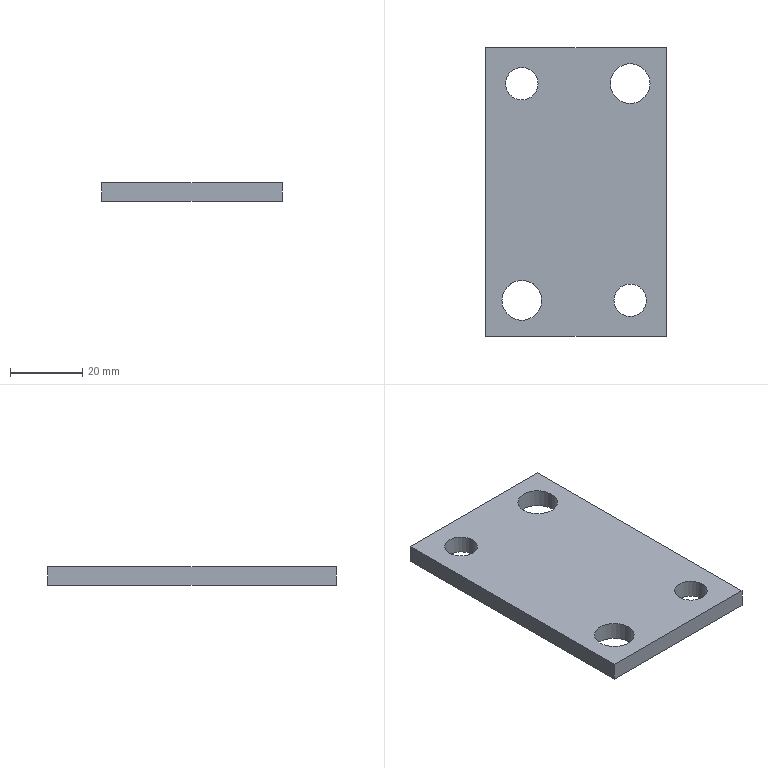Part | NX | features solid 2 | 1 solid | 10 faces | box 50 x 80 x 5 mm | volume 18413 mm3 | plane 6 | cylinder 4 | commonest cylinder face diameters 9 x2 11 x2
STEP:
#1=CARTESIAN_POINT('',(-560.,220.,154.));
#2=VERTEX_POINT('',#1);
#3=CARTESIAN_POINT('',(-560.,140.,154.));
#4=VERTEX_POINT('',#3);
#5=CARTESIAN_POINT('',(-560.,169.049,154.));
#6=DIRECTION('',(0.,1.,0.));
#7=VECTOR('',#6,1000.);
#8=LINE('',#5,#7);
#9=EDGE_CURVE('',#2,#4,#8,.F.);
#10=ORIENTED_EDGE('',*,*,#9,.T.);
#11=CARTESIAN_POINT('',(-560.,140.,159.));
#12=VERTEX_POINT('',#11);
#13=CARTESIAN_POINT('',(-560.,140.,159.));
#14=DIRECTION('',(0.,0.,-1.));
#15=VECTOR('',#14,1000.);
#16=LINE('',#13,#15);
#17=EDGE_CURVE('',#12,#4,#16,.T.);
#18=ORIENTED_EDGE('',*,*,#17,.F.);
#19=CARTESIAN_POINT('',(-560.,220.,159.));
#20=VERTEX_POINT('',#19);
#21=CARTESIAN_POINT('',(-560.,169.049,159.));
#22=DIRECTION('',(0.,1.,0.));
#23=VECTOR('',#22,1000.);
#24=LINE('',#21,#23);
#25=EDGE_CURVE('',#20,#12,#24,.F.);
#26=ORIENTED_EDGE('',*,*,#25,.F.);
#27=CARTESIAN_POINT('',(-560.,220.,159.));
#28=DIRECTION('',(0.,0.,-1.));
#29=VECTOR('',#28,1000.);
#30=LINE('',#27,#29);
#31=EDGE_CURVE('',#20,#2,#30,.T.);
#32=ORIENTED_EDGE('',*,*,#31,.T.);
#33=EDGE_LOOP('',(#10,#18,#26,#32));
#34=FACE_BOUND('',#33,.T.);
#35=CARTESIAN_POINT('',(-560.,169.049,159.));
#36=DIRECTION('',(1.,0.,0.));
#37=DIRECTION('',(0.,0.,-1.));
#38=AXIS2_PLACEMENT_3D('',#35,#36,#37);
#39=PLANE('',#38);
#40=ADVANCED_FACE('',(#34),#39,.F.);
#41=CARTESIAN_POINT('',(-510.,140.,154.));
#42=VERTEX_POINT('',#41);
#43=CARTESIAN_POINT('',(-542.438,140.,154.));
#44=DIRECTION('',(-1.,0.,0.));
#45=VECTOR('',#44,1000.);
#46=LINE('',#43,#45);
#47=EDGE_CURVE('',#4,#42,#46,.F.);
#48=ORIENTED_EDGE('',*,*,#47,.T.);
#49=CARTESIAN_POINT('',(-510.,140.,159.));
#50=VERTEX_POINT('',#49);
#51=CARTESIAN_POINT('',(-510.,140.,159.));
#52=DIRECTION('',(0.,0.,-1.));
#53=VECTOR('',#52,1000.);
#54=LINE('',#51,#53);
#55=EDGE_CURVE('',#50,#42,#54,.T.);
#56=ORIENTED_EDGE('',*,*,#55,.F.);
#57=CARTESIAN_POINT('',(-542.438,140.,159.));
#58=DIRECTION('',(-1.,0.,0.));
#59=VECTOR('',#58,1000.);
#60=LINE('',#57,#59);
#61=EDGE_CURVE('',#12,#50,#60,.F.);
#62=ORIENTED_EDGE('',*,*,#61,.F.);
#63=ORIENTED_EDGE('',*,*,#17,.T.);
#64=EDGE_LOOP('',(#48,#56,#62,#63));
#65=FACE_BOUND('',#64,.T.);
#66=CARTESIAN_POINT('',(-542.438,140.,159.));
#67=DIRECTION('',(0.,1.,0.));
#68=DIRECTION('',(0.,0.,1.));
#69=AXIS2_PLACEMENT_3D('',#66,#67,#68);
#70=PLANE('',#69);
#71=ADVANCED_FACE('',(#65),#70,.F.);
#72=CARTESIAN_POINT('',(-510.,220.,154.));
#73=VERTEX_POINT('',#72);
#74=CARTESIAN_POINT('',(-510.,169.049,154.));
#75=DIRECTION('',(0.,-1.,0.));
#76=VECTOR('',#75,1000.);
#77=LINE('',#74,#76);
#78=EDGE_CURVE('',#42,#73,#77,.F.);
#79=ORIENTED_EDGE('',*,*,#78,.T.);
#80=CARTESIAN_POINT('',(-510.,220.,159.));
#81=VERTEX_POINT('',#80);
#82=CARTESIAN_POINT('',(-510.,220.,159.));
#83=DIRECTION('',(0.,0.,-1.));
#84=VECTOR('',#83,1000.);
#85=LINE('',#82,#84);
#86=EDGE_CURVE('',#81,#73,#85,.T.);
#87=ORIENTED_EDGE('',*,*,#86,.F.);
#88=CARTESIAN_POINT('',(-510.,169.049,159.));
#89=DIRECTION('',(0.,-1.,0.));
#90=VECTOR('',#89,1000.);
#91=LINE('',#88,#90);
#92=EDGE_CURVE('',#50,#81,#91,.F.);
#93=ORIENTED_EDGE('',*,*,#92,.F.);
#94=ORIENTED_EDGE('',*,*,#55,.T.);
#95=EDGE_LOOP('',(#79,#87,#93,#94));
#96=FACE_BOUND('',#95,.T.);
#97=CARTESIAN_POINT('',(-510.,169.049,159.));
#98=DIRECTION('',(-1.,0.,0.));
#99=DIRECTION('',(0.,0.,1.));
#100=AXIS2_PLACEMENT_3D('',#97,#98,#99);
#101=PLANE('',#100);
#102=ADVANCED_FACE('',(#96),#101,.F.);
#103=CARTESIAN_POINT('',(-515.5,150.,159.));
#104=VERTEX_POINT('',#103);
#105=CARTESIAN_POINT('',(-520.,150.,159.));
#106=DIRECTION('',(0.,0.,1.));
#107=DIRECTION('',(1.,0.,0.));
#108=AXIS2_PLACEMENT_3D('',#105,#106,#107);
#109=CIRCLE('',#108,4.5);
#110=EDGE_CURVE('',#104,#104,#109,.T.);
#111=ORIENTED_EDGE('',*,*,#110,.T.);
#112=EDGE_LOOP('',(#111));
#113=FACE_BOUND('',#112,.T.);
#114=CARTESIAN_POINT('',(-515.5,150.,154.));
#115=VERTEX_POINT('',#114);
#116=CARTESIAN_POINT('',(-520.,150.,154.));
#117=DIRECTION('',(0.,0.,1.));
#118=DIRECTION('',(1.,0.,0.));
#119=AXIS2_PLACEMENT_3D('',#116,#117,#118);
#120=CIRCLE('',#119,4.5);
#121=EDGE_CURVE('',#115,#115,#120,.T.);
#122=ORIENTED_EDGE('',*,*,#121,.F.);
#123=EDGE_LOOP('',(#122));
#124=FACE_BOUND('',#123,.T.);
#125=CARTESIAN_POINT('',(-520.,150.,159.));
#126=DIRECTION('',(0.,0.,-1.));
#127=DIRECTION('',(-1.,0.,0.));
#128=AXIS2_PLACEMENT_3D('',#125,#126,#127);
#129=CYLINDRICAL_SURFACE('',#128,4.5);
#130=ADVANCED_FACE('',(#113,#124),#129,.F.);
#131=CARTESIAN_POINT('',(-545.5,210.,159.));
#132=VERTEX_POINT('',#131);
#133=CARTESIAN_POINT('',(-550.,210.,159.));
#134=DIRECTION('',(0.,0.,1.));
#135=DIRECTION('',(1.,0.,0.));
#136=AXIS2_PLACEMENT_3D('',#133,#134,#135);
#137=CIRCLE('',#136,4.5);
#138=EDGE_CURVE('',#132,#132,#137,.T.);
#139=ORIENTED_EDGE('',*,*,#138,.T.);
#140=EDGE_LOOP('',(#139));
#141=FACE_BOUND('',#140,.T.);
#142=CARTESIAN_POINT('',(-545.5,210.,154.));
#143=VERTEX_POINT('',#142);
#144=CARTESIAN_POINT('',(-550.,210.,154.));
#145=DIRECTION('',(0.,0.,1.));
#146=DIRECTION('',(1.,0.,0.));
#147=AXIS2_PLACEMENT_3D('',#144,#145,#146);
#148=CIRCLE('',#147,4.5);
#149=EDGE_CURVE('',#143,#143,#148,.T.);
#150=ORIENTED_EDGE('',*,*,#149,.F.);
#151=EDGE_LOOP('',(#150));
#152=FACE_BOUND('',#151,.T.);
#153=CARTESIAN_POINT('',(-550.,210.,159.));
#154=DIRECTION('',(0.,0.,-1.));
#155=DIRECTION('',(-1.,0.,0.));
#156=AXIS2_PLACEMENT_3D('',#153,#154,#155);
#157=CYLINDRICAL_SURFACE('',#156,4.5);
#158=ADVANCED_FACE('',(#141,#152),#157,.F.);
#159=CARTESIAN_POINT('',(-544.5,150.,159.));
#160=VERTEX_POINT('',#159);
#161=CARTESIAN_POINT('',(-550.,150.,159.));
#162=DIRECTION('',(0.,0.,1.));
#163=DIRECTION('',(1.,0.,0.));
#164=AXIS2_PLACEMENT_3D('',#161,#162,#163);
#165=CIRCLE('',#164,5.5);
#166=EDGE_CURVE('',#160,#160,#165,.T.);
#167=ORIENTED_EDGE('',*,*,#166,.T.);
#168=EDGE_LOOP('',(#167));
#169=FACE_BOUND('',#168,.T.);
#170=CARTESIAN_POINT('',(-544.5,150.,154.));
#171=VERTEX_POINT('',#170);
#172=CARTESIAN_POINT('',(-550.,150.,154.));
#173=DIRECTION('',(0.,0.,1.));
#174=DIRECTION('',(1.,0.,0.));
#175=AXIS2_PLACEMENT_3D('',#172,#173,#174);
#176=CIRCLE('',#175,5.5);
#177=EDGE_CURVE('',#171,#171,#176,.T.);
#178=ORIENTED_EDGE('',*,*,#177,.F.);
#179=EDGE_LOOP('',(#178));
#180=FACE_BOUND('',#179,.T.);
#181=CARTESIAN_POINT('',(-550.,150.,159.));
#182=DIRECTION('',(0.,0.,-1.));
#183=DIRECTION('',(-1.,0.,0.));
#184=AXIS2_PLACEMENT_3D('',#181,#182,#183);
#185=CYLINDRICAL_SURFACE('',#184,5.5);
#186=ADVANCED_FACE('',(#169,#180),#185,.F.);
#187=CARTESIAN_POINT('',(-514.5,210.,159.));
#188=VERTEX_POINT('',#187);
#189=CARTESIAN_POINT('',(-520.,210.,159.));
#190=DIRECTION('',(0.,0.,1.));
#191=DIRECTION('',(1.,0.,0.));
#192=AXIS2_PLACEMENT_3D('',#189,#190,#191);
#193=CIRCLE('',#192,5.5);
#194=EDGE_CURVE('',#188,#188,#193,.T.);
#195=ORIENTED_EDGE('',*,*,#194,.T.);
#196=EDGE_LOOP('',(#195));
#197=FACE_BOUND('',#196,.T.);
#198=CARTESIAN_POINT('',(-514.5,210.,154.));
#199=VERTEX_POINT('',#198);
#200=CARTESIAN_POINT('',(-520.,210.,154.));
#201=DIRECTION('',(0.,0.,1.));
#202=DIRECTION('',(1.,0.,0.));
#203=AXIS2_PLACEMENT_3D('',#200,#201,#202);
#204=CIRCLE('',#203,5.5);
#205=EDGE_CURVE('',#199,#199,#204,.T.);
#206=ORIENTED_EDGE('',*,*,#205,.F.);
#207=EDGE_LOOP('',(#206));
#208=FACE_BOUND('',#207,.T.);
#209=CARTESIAN_POINT('',(-520.,210.,159.));
#210=DIRECTION('',(0.,0.,-1.));
#211=DIRECTION('',(-1.,0.,0.));
#212=AXIS2_PLACEMENT_3D('',#209,#210,#211);
#213=CYLINDRICAL_SURFACE('',#212,5.5);
#214=ADVANCED_FACE('',(#197,#208),#213,.F.);
#215=CARTESIAN_POINT('',(-542.438,220.,154.));
#216=DIRECTION('',(1.,0.,0.));
#217=VECTOR('',#216,1000.);
#218=LINE('',#215,#217);
#219=EDGE_CURVE('',#73,#2,#218,.F.);
#220=ORIENTED_EDGE('',*,*,#219,.T.);
#221=ORIENTED_EDGE('',*,*,#31,.F.);
#222=CARTESIAN_POINT('',(-542.438,220.,159.));
#223=DIRECTION('',(1.,0.,0.));
#224=VECTOR('',#223,1000.);
#225=LINE('',#222,#224);
#226=EDGE_CURVE('',#81,#20,#225,.F.);
#227=ORIENTED_EDGE('',*,*,#226,.F.);
#228=ORIENTED_EDGE('',*,*,#86,.T.);
#229=EDGE_LOOP('',(#220,#221,#227,#228));
#230=FACE_BOUND('',#229,.T.);
#231=CARTESIAN_POINT('',(-542.438,220.,159.));
#232=DIRECTION('',(0.,-1.,0.));
#233=DIRECTION('',(0.,0.,-1.));
#234=AXIS2_PLACEMENT_3D('',#231,#232,#233);
#235=PLANE('',#234);
#236=ADVANCED_FACE('',(#230),#235,.F.);
#237=ORIENTED_EDGE('',*,*,#194,.F.);
#238=EDGE_LOOP('',(#237));
#239=FACE_BOUND('',#238,.T.);
#240=ORIENTED_EDGE('',*,*,#166,.F.);
#241=EDGE_LOOP('',(#240));
#242=FACE_BOUND('',#241,.T.);
#243=ORIENTED_EDGE('',*,*,#138,.F.);
#244=EDGE_LOOP('',(#243));
#245=FACE_BOUND('',#244,.T.);
#246=ORIENTED_EDGE('',*,*,#110,.F.);
#247=EDGE_LOOP('',(#246));
#248=FACE_BOUND('',#247,.T.);
#249=ORIENTED_EDGE('',*,*,#25,.T.);
#250=ORIENTED_EDGE('',*,*,#61,.T.);
#251=ORIENTED_EDGE('',*,*,#92,.T.);
#252=ORIENTED_EDGE('',*,*,#226,.T.);
#253=EDGE_LOOP('',(#249,#250,#251,#252));
#254=FACE_BOUND('',#253,.T.);
#255=CARTESIAN_POINT('',(-542.438,169.049,159.));
#256=DIRECTION('',(0.,0.,1.));
#257=DIRECTION('',(1.,0.,0.));
#258=AXIS2_PLACEMENT_3D('',#255,#256,#257);
#259=PLANE('',#258);
#260=ADVANCED_FACE('',(#239,#242,#245,#248,#254),#259,.T.);
#261=ORIENTED_EDGE('',*,*,#205,.T.);
#262=EDGE_LOOP('',(#261));
#263=FACE_BOUND('',#262,.T.);
#264=ORIENTED_EDGE('',*,*,#177,.T.);
#265=EDGE_LOOP('',(#264));
#266=FACE_BOUND('',#265,.T.);
#267=ORIENTED_EDGE('',*,*,#149,.T.);
#268=EDGE_LOOP('',(#267));
#269=FACE_BOUND('',#268,.T.);
#270=ORIENTED_EDGE('',*,*,#121,.T.);
#271=EDGE_LOOP('',(#270));
#272=FACE_BOUND('',#271,.T.);
#273=ORIENTED_EDGE('',*,*,#9,.F.);
#274=ORIENTED_EDGE('',*,*,#219,.F.);
#275=ORIENTED_EDGE('',*,*,#78,.F.);
#276=ORIENTED_EDGE('',*,*,#47,.F.);
#277=EDGE_LOOP('',(#273,#274,#275,#276));
#278=FACE_BOUND('',#277,.T.);
#279=CARTESIAN_POINT('',(-542.438,169.049,154.));
#280=DIRECTION('',(0.,0.,1.));
#281=DIRECTION('',(1.,0.,0.));
#282=AXIS2_PLACEMENT_3D('',#279,#280,#281);
#283=PLANE('',#282);
#284=ADVANCED_FACE('',(#263,#266,#269,#272,#278),#283,.F.);
#285=CLOSED_SHELL('',(#40,#71,#102,#130,#158,#186,#214,#236,#260,#284));
#286=MANIFOLD_SOLID_BREP('',#285);
#287=(LENGTH_UNIT()NAMED_UNIT(*)SI_UNIT(.MILLI.,.METRE.));
#288=UNCERTAINTY_MEASURE_WITH_UNIT(LENGTH_MEASURE(0.00001),#287,'','');
#289=(NAMED_UNIT(*)PLANE_ANGLE_UNIT()SI_UNIT($,.RADIAN.));
#290=(NAMED_UNIT(*)SI_UNIT($,.STERADIAN.)SOLID_ANGLE_UNIT());
#291=(GEOMETRIC_REPRESENTATION_CONTEXT(3)GLOBAL_UNCERTAINTY_ASSIGNED_CONTEXT((#288))GLOBAL_UNIT_ASSIGNED_CONTEXT((#287,#289,#290))REPRESENTATION_CONTEXT('',''));
#292=ADVANCED_BREP_SHAPE_REPRESENTATION('',(#286),#291);